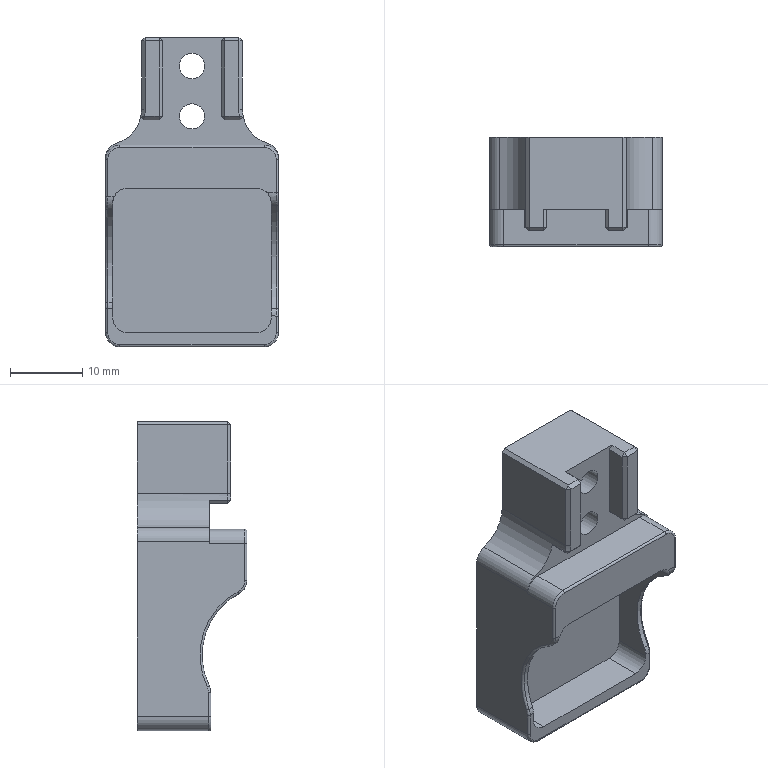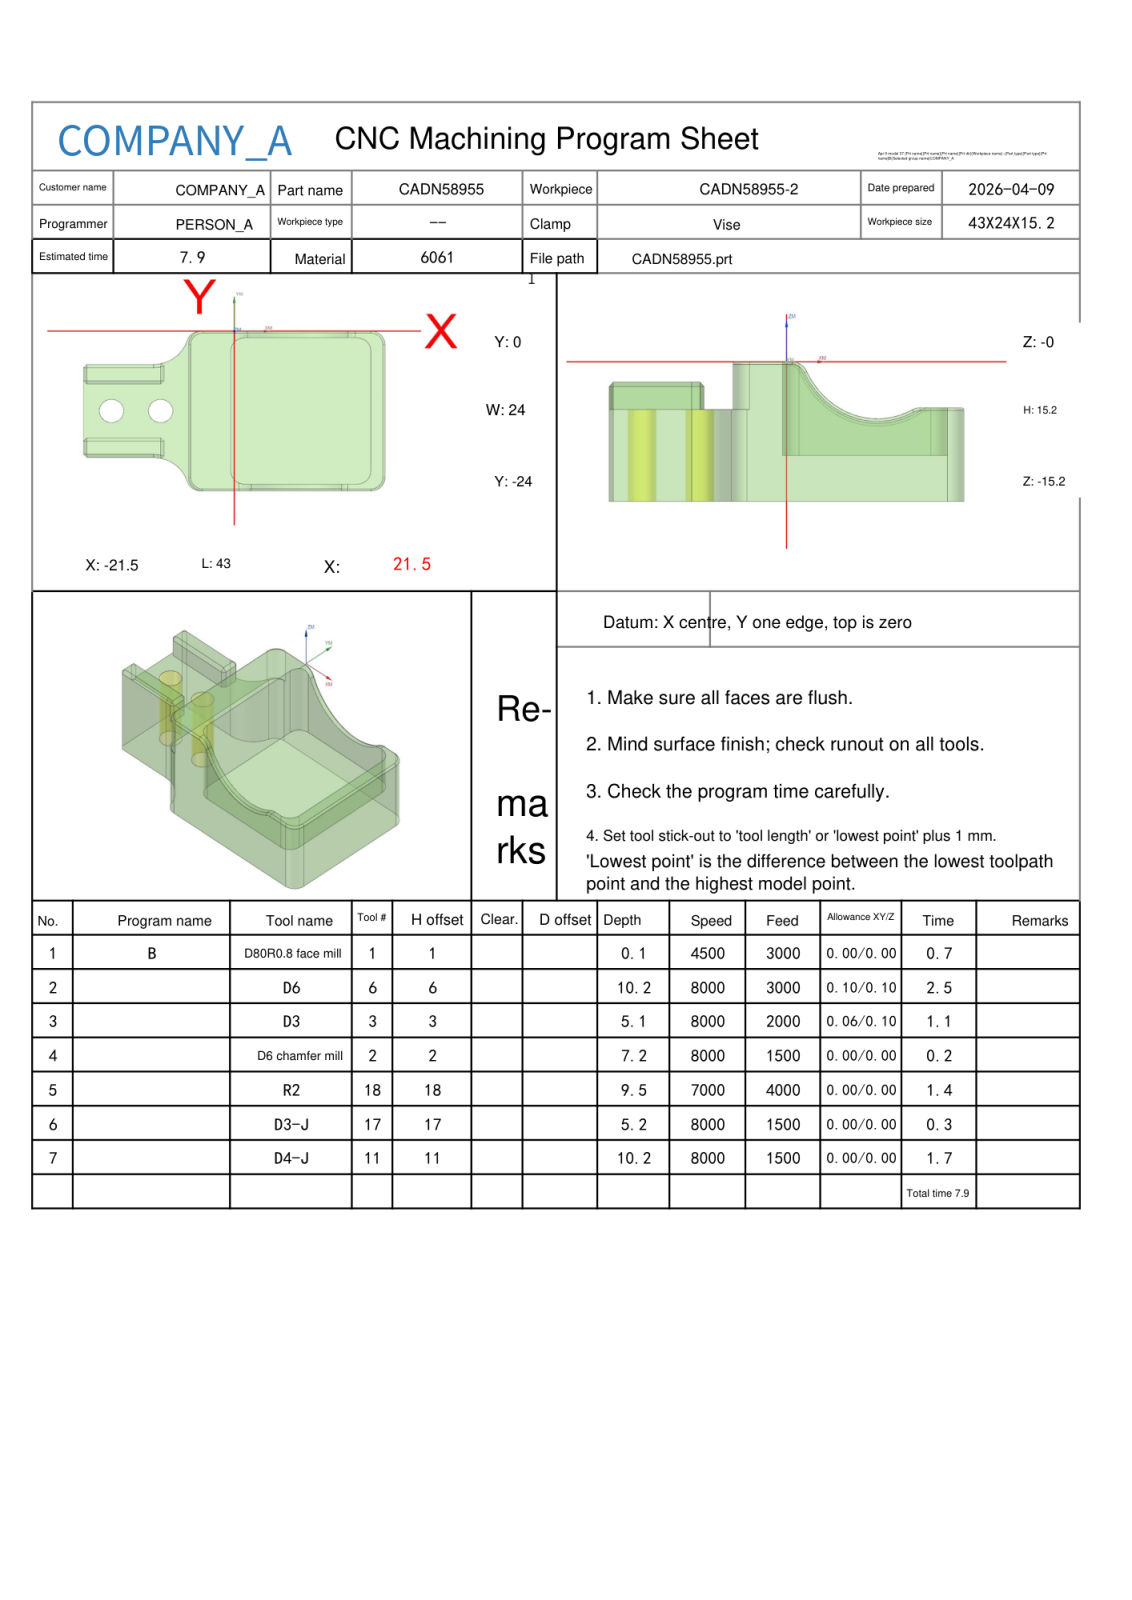NC program | NX | posted by the shop | part box 24 x 15.2 x 43 mm
Lines 3234 to 4724 of 14472:
N5 T18 M06
(R2  D=4. R=2. H=18 ce=0.01 di=0.00)
G00 G90 G54 X3.945 Y-24.084 M03 S7000
G43 H18 Z14.5
M08
Z.491
G01 Z-.009 F4000.
X1.773 Y-23.864
X1.579 Y-23.845
X.675 Y-23.917
X-4.5
G02 X-6.417 Y-22. I0.0 J1.917
G01 Y-2.
G02 X-4.5 Y-.083 I1.917 J0.0
G01 X.099
X1.018 Y-.155
X1.197 Y-.136
X1.199 Y-.039 Z-.016
Y.003 Z-.022
X.175 Y.009
X.099 Y.028
X-4.5
G03 X-6.528 Y-2. I0.0 J-2.028
G01 Y-22.
G03 X-4.5 Y-24.028 I2.028 J0.0
G01 X.675
X.737 Y-24.01
X1.774 Y-23.998
Y-24.071 Z-.031
Y-24.091 Z-.039
X.737 Y-24.103
X.675 Y-24.132
X-4.5
G02 X-6.632 Y-22. I0.0 J2.132
G01 Y-2.
G02 X-4.5 Y.132 I2.132 J0.0
G01 X.099
X.175 Y.103
X1.199 Y.1
Y.174 Z-.05
Y.216 Z-.06
X.175 Y.22
X.099 Y.233
X-4.5
G03 X-6.733 Y-2. I0.0 J-2.233
G01 Y-22.
G03 X-4.5 Y-24.233 I2.233 J0.0
G01 X.675
X.737 Y-24.22
X1.774 Y-24.208
Y-24.275 Z-.073
Y-24.313 Z-.086
X.737 Y-24.32
X.675 Y-24.333
X-4.5
G02 X-6.833 Y-22. I0.0 J2.333
G01 Y-2.
G02 X-4.5 Y.333 I2.333 J0.0
G01 X.099
X.175 Y.32
X1.199 Y.312
Y.374 Z-.101
Y.406 Z-.116
X.175 Y.414
X.099 Y.43
X-4.5
G03 X-6.93 Y-2. I0.0 J-2.43
G01 Y-22.
G03 X-4.5 Y-24.43 I2.43 J0.0
G01 X.675
X.737 Y-24.414
X1.774 Y-24.407
Y-24.471 Z-.133
Y-24.513 Z-.149
X.737 Y-24.52
X.675 Y-24.526
X-4.5
G02 X-7.026 Y-22. I0.0 J2.526
G01 Y-2.
G02 X-4.5 Y.526 I2.526 J0.0
G01 X.099
X.175 Y.52
X1.199 Y.512
Y.568 Z-.168
Y.603 Z-.187
X.175 Y.609
X.099 Y.619
X-4.5
G03 X-7.119 Y-2. I0.0 J-2.619
G01 Y-22.
G03 X-4.5 Y-24.619 I2.619 J0.0
G01 X.675
X.737 Y-24.609
X1.774 Y-24.604
Y-24.661 Z-.208
Y-24.692 Z-.229
X.737 Y-24.698
X.675 Y-24.711
X-4.5
G02 X-7.211 Y-22. I0.0 J2.711
G01 Y-2.
G02 X-4.5 Y.711 I2.711 J0.0
G01 X.099
X.175 Y.697
X1.199 Y.691
Y.75 Z-.252
Y.788 Z-.275
X1.018 Y.791
X.175 Y.793
X.099 Y.801
X-4.5
G03 X-7.301 Y-2. I0.0 J-2.801
G01 Y-22.
G03 X-4.5 Y-24.801 I2.801 J0.0
G01 X.675
X.737 Y-24.794
X1.774 Y-24.788
X1.719 Y-24.881 Z-.325
X.737 Y-24.879
X.675 Y-24.888
X-4.5
G02 X-7.388 Y-22. I0.0 J2.888
G01 Y-2.
G02 X-4.5 Y.888 I2.888 J0.0
G01 X.099
X.175 Y.884
X1.018 Y.882
X1.199 Y.879
Y.929 Z-.351
X1.2 Y.968 Z-.378
X1.018 Y.971
X.099 Y.973
X-4.5
G03 X-7.473 Y-2. I0.0 J-2.973
G01 Y-22.
G03 X-4.5 Y-24.973 I2.973 J0.0
G01 X.675
X1.779 Y-24.971
X1.788 Y-25.012 Z-.407
X1.798 Y-25.054 Z-.435
X.737 Y-25.047
X.675 Y-25.056
X-4.5
G02 X-7.556 Y-22. I0.0 J3.056
G01 Y-2.
G02 X-4.5 Y1.056 I3.056 J0.0
G01 X.099
X.175 Y1.052
X1.018 Y1.051
X1.199 Y1.048
Y1.094 Z-.465
Y1.132 Z-.495
X.175 Y1.133
X.099 Y1.136
X-4.5
G03 X-7.636 Y-2. I0.0 J-3.136
G01 Y-22.
G03 X-4.5 Y-25.136 I3.136 J0.0
G01 X.675
X.737 Y-25.133
X1.774
Y-25.172 Z-.527
Y-25.209 Z-.559
X.675 Y-25.213
X-4.5
G02 X-7.713 Y-22. I0.0 J3.213
G01 Y-2.
G02 X-4.5 Y1.213 I3.213 J0.0
G01 X.099
X.175 Y1.21
X1.202 Y1.208
X1.201 Y1.249 Z-.593
X1.199 Y1.285 Z-.627
X1.177 Y1.284
X.175 Y1.285
X.099 Y1.288
X-4.5
G03 X-7.788 Y-2. I0.0 J-3.288
G01 Y-22.
G03 X-4.5 Y-25.288 I3.288 J0.0
G01 X.675
X.737 Y-25.285
X1.7 Y-25.284
X1.784 Y-25.281
X1.779 Y-25.323 Z-.662
X1.775 Y-25.357 Z-.697
X1.712 Y-25.355
X.737 Y-25.356
X.675 Y-25.359
X-4.5
G02 X-7.859 Y-22. I0.0 J3.359
G01 Y-2.
G02 X-4.5 Y1.359 I3.359 J0.0
G01 X.099
X.175 Y1.356
X1.199
Y1.391 Z-.734
Y1.424 Z-.77
X1.125 Y1.423
X.175 Y1.424
X.099 Y1.428
X-4.5
G03 X-7.928 Y-2. I0.0 J-3.428
G01 Y-22.
G03 X-4.5 Y-25.428 I3.428 J0.0
G01 X.675
X.737 Y-25.425
X1.775 Y-25.423
Y-25.457 Z-.808
Y-25.487 Z-.847
X.737 Y-25.489
X.675 Y-25.493
X-4.5
G02 X-7.993 Y-22. I0.0 J3.493
G01 Y-2.
G02 X-4.5 Y1.493 I3.493 J0.0
G01 X.099
X.175 Y1.489
X1.199 Y1.488
Y1.521 Z-.886
Y1.551 Z-.926
X1.142 Y1.55
X.175 Y1.551
X.099 Y1.554
X-4.5
G03 X-8.054 Y-2. I0.0 J-3.554
G01 Y-22.
G03 X-4.5 Y-25.554 I3.554 J0.0
G01 X.675
X.737 Y-25.551
X1.704 Y-25.55
X1.775 Y-25.552
Y-25.582 Z-.966
Y-25.607 Z-1.007
X1.712 Y-25.606
X.737 Y-25.607
X.675 Y-25.612
X-4.5
G02 X-8.112 Y-22. I0.0 J3.612
G01 Y-2.
G02 X-4.5 Y1.612 I3.612 J0.0
G01 X.099
X.175 Y1.607
X1.15 Y1.606
X1.199 Y1.607
Y1.639 Z-1.049
X1.2 Y1.664 Z-1.091
X.175 Y1.665
X.099 Y1.667
X-4.5
G03 X-8.167 Y-2. I0.0 J-3.667
G01 Y-22.
G03 X-4.5 Y-25.667 I3.667 J0.0
G01 X.675
X.737 Y-25.665
X1.775 Y-25.664
Y-25.691 Z-1.134
X1.774 Y-25.713 Z-1.177
X1.7 Y-25.711
X.737 Y-25.713
X.675 Y-25.717
X-4.5
G02 X-8.217 Y-22. I0.0 J3.717
G01 Y-2.
G02 X-4.5 Y1.717 I3.717 J0.0
G01 X.099
X.175 Y1.712
X1.2 Y1.714
Y1.738 Z-1.222
Y1.761 Z-1.266
X.175 Y1.759
X.099 Y1.764
X-4.5
G03 X-8.264 Y-2. I0.0 J-3.764
G01 Y-22.
G03 X-4.5 Y-25.764 I3.764 J0.0
G01 X.675
X.737 Y-25.759
X1.775 Y-25.758
Y-25.785 Z-1.311
Y-25.803 Z-1.356
X1.708 Y-25.804
X.737 Y-25.806
X.675 Y-25.807
X-4.5
G02 X-8.307 Y-22. I0.0 J3.807
G01 Y-2.
G02 X-4.5 Y1.807 I3.807 J0.0
G01 X.099
X.175 Y1.806
X1.2 Y1.805
Y1.824 Z-1.402
Y1.842 Z-1.448
X1.154 Y1.843
X.175 Y1.844
X.099 Y1.847
X-4.5
G03 X-8.347 Y-2. I0.0 J-3.847
G01 Y-22.
G03 X-4.5 Y-25.847 I3.847 J0.0
G01 X.675
X.737 Y-25.844
X1.711 Y-25.843
X1.775
Y-25.863 Z-1.495
Y-25.878 Z-1.542
X.737 Y-25.88
X.675 Y-25.882
X-4.5
G02 X-8.382 Y-22. I0.0 J3.882
G01 Y-2.
G02 X-4.5 Y1.882 I3.882 J0.0
G01 X.099
X.175 Y1.88
X1.158 Y1.879
X1.2 Y1.878
Y1.894 Z-1.59
Y1.907 Z-1.637
X1.156 Y1.908
X.175
X.099 Y1.912
X-4.5
G03 X-8.412 Y-2. I0.0 J-3.912
G01 Y-22.
G03 X-4.5 Y-25.912 I3.912 J0.0
G01 X.675
X.737 Y-25.908
X1.717
X1.775
Y-25.922 Z-1.685
Y-25.935 Z-1.734
X.737 Y-25.936
X.675 Y-25.939
X-4.5
G02 X-8.439 Y-22. I0.0 J3.939
G01 Y-2.
G02 X-4.5 Y1.939 I3.939 J0.0
G01 X.099
X.175 Y1.935
X1.158 Y1.934
X1.2
X1.201 Y1.949 Z-1.782
X1.202 Y1.96 Z-1.831
X.175 Y1.961
X.099 Y1.962
X-4.5
G03 X-8.462 Y-2. I0.0 J-3.962
G01 Y-22.
G03 X-4.5 Y-25.962 I3.962 J0.0
G01 X.675
X.737 Y-25.961
X1.781 Y-25.96
Y-25.97 Z-1.88
Y-25.978 Z-1.929
X.737 Y-25.979
X.675 Y-25.98
X-4.5
G02 X-8.48 Y-22. I0.0 J3.98
G01 Y-2.
G02 X-4.5 Y1.98 I3.98 J0.0
G01 X.099
X.175 Y1.979
X1.202 Y1.978
Y1.984 Z-1.976
Y1.989 Z-2.022
X.175
X.099 Y1.993
X-4.5
G03 X-8.493 Y-2. I0.0 J-3.993
G01 Y-22.
G03 X-4.5 Y-25.993 I3.993 J0.0
G01 X.675
X.737 Y-25.989
X1.781
Y-25.997 Z-2.115
X.737 Y-25.998
X.675 Y-26.003
X-4.5
G02 X-8.503 Y-22. I0.0 J4.003
G01 Y-2.
G02 X-4.5 Y2.003 I4.003 J0.0
G01 X.099
X.175 Y1.998
X1.202 Y1.997
Y2.006 Z-2.207
X.175
X.099 Y2.008
X-4.5
G03 X-8.508 Y-2. I0.0 J-4.008
G01 Y-22.
G03 X-4.5 Y-26.008 I4.008 J0.0
G01 X.675
X.737 Y-26.006
X1.781
Y-26.01 Z-2.3
X-4.529 Y-26.009
G02 X-4.744 Y-26.003 I0.0 J3.532
X-8.25 Y-23.42 I.244 J4.003
X-8.51 Y-22. I3.75 J1.42
G01 Y-2.
G02 X-8.25 Y-.58 I4.01 J0.0
X-4.878 Y1.992 I3.75 J-1.42
G01 X-4.5 Y2.01
X1.202
G00 Z14.5
G00 G90 X13.988 Y-.296 M03 S7000
Z14.5
Z-4.509
G01 Z-5.009 F4000.
X16.131 Y-.155
X17.231 Y-.083
X19.5
G02 X21.417 Y-2. I0.0 J-1.917
G01 Y-22.
G02 X19.5 Y-23.917 I-1.917 J0.0
G01 X16.159
X15.277 Y-23.845
X15.063 Y-23.878
X15.06 Y-23.961 Z-5.016
X15.059 Y-24. Z-5.022
X16.123 Y-24.013
X16.159 Y-24.028
X19.5
G03 X21.528 Y-22. I0.0 J2.028
G01 Y-2.
G03 X19.5 Y.028 I-2.028 J0.0
G01 X17.231
X16.131 Y.004
Y.07 Z-5.031
Y.098 Z-5.039
X17.231 Y.132
X19.5
G02 X21.632 Y-2. I0.0 J-2.132
G01 Y-22.
G02 X19.5 Y-24.132 I-2.132 J0.0
G01 X16.159
X15.059 Y-24.093
Y-24.21 Z-5.06
X16.123 Y-24.222
X16.159 Y-24.233
X19.5
G03 X21.733 Y-22. I0.0 J2.233
G01 Y-2.
G03 X19.5 Y.233 I-2.233 J0.0
G01 X17.231
X16.131 Y.215
Y.275 Z-5.073
Y.317 Z-5.086
X17.231 Y.333
X19.5
G02 X21.833 Y-2. I0.0 J-2.333
G01 Y-22.
G02 X19.5 Y-24.333 I-2.333 J0.0
G01 X16.159
X16.123 Y-24.321
X15.108
X15.03 Y-24.32
X15.057 Y-24.42 Z-5.116
X15.104 Y-24.412
X16.123 Y-24.414
X16.159 Y-24.43
X19.5
G03 X21.93 Y-22. I0.0 J2.43
G01 Y-2.
G03 X19.5 Y.43 I-2.43 J0.0
G01 X17.231
X16.131 Y.411
Y.471 Z-5.133
Y.517 Z-5.149
X17.231 Y.526
X19.5
G02 X22.026 Y-2. I0.0 J-2.526
G01 Y-22.
G02 X19.5 Y-24.526 I-2.526 J0.0
G01 X16.159
X16.123 Y-24.521
X15.05 Y-24.52
X15.055 Y-24.571 Z-5.168
X15.059 Y-24.616 Z-5.187
X16.159 Y-24.619
X19.5
G03 X22.119 Y-22. I0.0 J2.619
G01 Y-2.
G03 X19.5 Y.619 I-2.619 J0.0
G01 X17.231
X16.131 Y.607
Y.661 Z-5.208
Y.695 Z-5.229
X17.231 Y.711
X19.5
G02 X22.211 Y-2. I0.0 J-2.711
G01 Y-22.
G02 X19.5 Y-24.711 I-2.711 J0.0
G01 X16.159
X16.123 Y-24.698
X15.059 Y-24.707
X15.055 Y-24.753 Z-5.252
X15.051 Y-24.796 Z-5.275
X16.123 Y-24.795
X16.159 Y-24.801
X19.5
G03 X22.301 Y-22. I0.0 J2.801
G01 Y-2.
G03 X19.5 Y.801 I-2.801 J0.0
G01 X17.231
X16.131 Y.791
Y.84 Z-5.3
Y.884 Z-5.325
X16.161 Y.882
X17.231 Y.888
X19.5
G02 X22.388 Y-2. I0.0 J-2.888
G01 Y-22.
G02 X19.5 Y-24.888 I-2.888 J0.0
G01 X16.159
X16.123 Y-24.88
X15.045 Y-24.882
Y-24.927 Z-5.351
Y-24.971 Z-5.378
X16.123 Y-24.961
X16.159 Y-24.973
X19.5
G03 X22.473 Y-22. I0.0 J2.973
G01 Y-2.
G03 X19.5 Y.973 I-2.973 J0.0
G01 X17.231
X16.123 Y.971
X16.127 Y1.014 Z-5.407
X16.131 Y1.052 Z-5.435
X17.231 Y1.056
X19.5
G02 X22.556 Y-2. I0.0 J-3.056
G01 Y-22.
G02 X19.5 Y-25.056 I-3.056 J0.0
G01 X16.159
X16.123 Y-25.048
X15.045 Y-25.051
X15.053 Y-25.094 Z-5.465
X15.059 Y-25.133 Z-5.495
X16.123 Y-25.134
X16.159 Y-25.136
X19.5
G03 X22.636 Y-22. I0.0 J3.136
G01 Y-2.
G03 X19.5 Y1.136 I-3.136 J0.0
G01 X17.231
X16.131 Y1.132
Y1.171 Z-5.527
Y1.209 Z-5.559
X17.231 Y1.213
X19.5
G02 X22.713 Y-2. I0.0 J-3.213
G01 Y-22.
G02 X19.5 Y-25.213 I-3.213 J0.0
G01 X16.159
X16.123 Y-25.211
X15.056 Y-25.208
X15.058 Y-25.249 Z-5.593
X15.059 Y-25.285 Z-5.627
X15.081 Y-25.284
X16.123 Y-25.285
X16.159 Y-25.288
X19.5
G03 X22.788 Y-22. I0.0 J3.288
G01 Y-2.
G03 X19.5 Y1.288 I-3.288 J0.0
G01 X17.231
X16.14 Y1.281
X16.131 Y1.285
Y1.323 Z-5.662
Y1.357 Z-5.697
X16.193 Y1.355
X17.231 Y1.359
X19.5
G02 X22.859 Y-2. I0.0 J-3.359
G01 Y-22.
G02 X19.5 Y-25.359 I-3.359 J0.0
G01 X16.159
X16.123 Y-25.357
X15.059 Y-25.355
Y-25.391 Z-5.734
Y-25.424 Z-5.77
X16.123 Y-25.425
X16.159 Y-25.428
X19.5
G03 X22.928 Y-22. I0.0 J3.428
G01 Y-2.
G03 X19.5 Y1.428 I-3.428 J0.0
G01 X17.231
X16.131 Y1.423
Y1.457 Z-5.808
Y1.487 Z-5.847
X17.231 Y1.493
X19.5
G02 X22.993 Y-2. I0.0 J-3.493
G01 Y-22.
G02 X19.5 Y-25.493 I-3.493 J0.0
G01 X16.159
X16.123 Y-25.489
X15.059
Y-25.52 Z-5.886
Y-25.551 Z-5.926
X16.123 Y-25.552
X16.159 Y-25.554
X19.5
G03 X23.054 Y-22. I0.0 J3.554
G01 Y-2.
G03 X19.5 Y1.554 I-3.554 J0.0
G01 X17.231
X16.131 Y1.55
Y1.581 Z-5.966
Y1.606 Z-6.007
X17.231 Y1.612
X19.5
G02 X23.112 Y-2. I0.0 J-3.612
G01 Y-22.
G02 X19.5 Y-25.612 I-3.612 J0.0
G01 X16.159
X16.123 Y-25.608
X15.059 Y-25.609
Y-25.637 Z-6.049
Y-25.664 Z-6.091
X16.159 Y-25.667
X19.5
G03 X23.167 Y-22. I0.0 J3.667
G01 Y-2.
G03 X19.5 Y1.667 I-3.667 J0.0
G01 X17.231
X16.131 Y1.664
Y1.689 Z-6.134
Y1.711 Z-6.177
X17.231 Y1.717
X19.5
G02 X23.217 Y-2. I0.0 J-3.717
G01 Y-22.
G02 X19.5 Y-25.717 I-3.717 J0.0
G01 X16.159
X16.123 Y-25.713
X15.059 Y-25.712
Y-25.739 Z-6.222
Y-25.758 Z-6.266
X16.123 Y-25.759
X16.159 Y-25.764
X19.5
G03 X23.264 Y-22. I0.0 J3.764
G01 Y-2.
G03 X19.5 Y1.764 I-3.764 J0.0
G01 X17.231
X16.131 Y1.757
Y1.783 Z-6.311
Y1.804 Z-6.356
X17.231 Y1.807
X19.5
G02 X23.307 Y-2. I0.0 J-3.807
G01 Y-22.
G02 X19.5 Y-25.807 I-3.807 J0.0
G01 X16.159
X16.123 Y-25.806
X15.058 Y-25.805
Y-25.824 Z-6.402
Y-25.843 Z-6.448
X16.123 Y-25.844
X16.159 Y-25.847
X19.5
G03 X23.347 Y-22. I0.0 J3.847
G01 Y-2.
G03 X19.5 Y1.847 I-3.847 J0.0
G01 X17.231
X16.131 Y1.843
Y1.861 Z-6.495
Y1.879 Z-6.542
X17.231 Y1.882
X19.5
G02 X23.382 Y-2. I0.0 J-3.882
G01 Y-22.
G02 X19.5 Y-25.882 I-3.882 J0.0
G01 X16.159
X15.277 Y-25.879
X15.058
Y-25.894 Z-6.59
X15.059 Y-25.908 Z-6.637
X16.123 Y-25.909
X16.159 Y-25.912
X19.5
G03 X23.412 Y-22. I0.0 J3.912
G01 Y-2.
G03 X19.5 Y1.912 I-3.912 J0.0
G01 X17.231
X16.131 Y1.908
Y1.922 Z-6.685
Y1.934 Z-6.734
X17.231 Y1.939
X19.5
G02 X23.439 Y-2. I0.0 J-3.939
G01 Y-22.
G02 X19.5 Y-25.939 I-3.939 J0.0
G01 X16.159
X16.123 Y-25.936
X15.059
X15.058 Y-25.949 Z-6.782
X15.057 Y-25.96 Z-6.831
X16.123 Y-25.961
X16.159 Y-25.962
X19.5
G03 X23.462 Y-22. I0.0 J3.962
G01 Y-2.
G03 X19.5 Y1.962 I-3.962 J0.0
G01 X17.231
X16.132 Y1.96
Y1.97 Z-6.88
Y1.978 Z-6.929
X17.231 Y1.98
X19.5
G02 X23.48 Y-2. I0.0 J-3.98
G01 Y-22.
G02 X19.5 Y-25.98 I-3.98 J0.0
G01 X16.159
X16.123 Y-25.979
X15.057 Y-25.978
Y-25.984 Z-6.976
Y-25.989 Z-7.022
X16.123
X16.159 Y-25.993
X19.5
G03 X23.493 Y-22. I0.0 J3.993
G01 Y-2.
G03 X19.5 Y1.993 I-3.993 J0.0
G01 X17.231
X16.132 Y1.99
Y1.999 Z-7.115
X17.231 Y2.003
X19.5
G02 X23.503 Y-2. I0.0 J-4.003
G01 Y-22.
G02 X19.5 Y-26.003 I-4.003 J0.0
G01 X16.159
X16.123 Y-25.998
X15.057 Y-25.997
Y-26.006 Z-7.207
X16.123
X16.159 Y-26.008
X19.5
G03 X23.508 Y-22. I0.0 J4.008
G01 Y-2.
G03 X19.5 Y2.008 I-4.008 J0.0
G01 X17.231
X16.132 Y2.007
Y2.009 Z-7.3
X19.508 Y2.01
G02 X23.51 Y-2. I-.008 J-4.01
G01 Y-22.
G02 X19.508 Y-26.01 I-4.01 J0.0
G01 X15.057
G00 Z14.5
G00 G90 X.164 Y-22.174 M03 S7000
Z20.
Z7.997
G01 Z-.003 F3500.
X.432
X.539 Y-22.214 Z-.005
X.741 Y-22.274 Z-.007
X.45 Z-.002
X.165 Z-.001
Y-22.371 Z0.0
X.54 Z-.003
X.848 Z-.009
X1.048 Z-.024
X1.172 Y-22.37 Z-.039
X1.247 Y-22.386 Z-.049
X1.517 Y-22.422 Z-.102
X1.645 Y-22.439 Z-.133
X1.845 Y-22.454 Z-.192
X2.044 Y-22.468 Z-.262
X2.113 Y-22.47 Z-.289
X2.045 Z-.262
X1.845 Z-.192
X1.645 Z-.132
X1.542 Z-.107
X1.247 Z-.048
X1.048 Z-.023
X.848 Z-.008
X.45 Z-.001
X.166 Z0.0
Z8.
G00 X3.417 Y-22.469
Z6.866
G01 Z-1.134
X3.439 Z-1.153
X3.543 Z-1.264
X3.638 Z-1.361
X3.838 Z-1.604
X4.037 Z-1.89
X4.435 Z-2.534
X4.843 Y-22.468 Z-3.117
X4.938 Z-3.243
X5.232 Z-3.591
X5.641 Z-4.016
X6.04 Z-4.376
X6.428 Z-4.686
X6.827 Z-4.967
X7.037 Y-22.467 Z-5.097
X7.225 Z-5.201
X7.624 Z-5.41
X7.812 Z-5.505
X8.022 Z-5.598
X8.421 Z-5.745
X8.82 Z-5.876
X9.218 Z-5.986
X9.804 Y-22.466 Z-6.102
X10.015 Z-6.132
X10.414 Z-6.17
X10.812 Z-6.18
X11.211 Z-6.183
X11.609 Z-6.168
X12.008 Y-22.465 Z-6.129
X12.407 Z-6.062
X12.805 Z-5.976
X13.204 Z-5.874
X13.416 Z-5.808
X14.001 Y-22.464 Z-5.592
X14.43 Z-5.412
X14.477 Z-5.394
X14.799 Y-22.47 Z-5.271
X14.894 Y-22.472 Z-5.237
X15.098 Y-22.476 Z-5.171
X15.196 Y-22.478 Z-5.141
X15.396 Y-22.484 Z-5.094
X15.595 Y-22.489 Z-5.06
X15.994 Y-22.502 Z-5.011
X16.392 Y-22.522 Z-5.
X16.668 Y-22.546 Z-5.002
X16.674 Y-22.547
X16.678 Y-22.556
X16.679 Y-22.562
X16.392 Y-22.563 Z-5.
X15.994 Z-5.01
X15.82 Z-5.029
X15.595 Z-5.057
X15.396 Z-5.091
X15.196 Z-5.138
X15.053 Z-5.18
X14.941 Z-5.217
X14.799 Z-5.267
X14.574 Z-5.353
X14.399 Z-5.423
X14.001 Y-22.564 Z-5.591
X13.602 Z-5.738
X13.426 Z-5.797
X13.315 Z-5.839
X13.204 Z-5.873
X12.805 Z-5.975
X12.407 Z-6.061
X12.008 Z-6.128
X11.609 Y-22.565 Z-6.166
X11.211 Z-6.183
X10.812 Z-6.18
X10.414 Z-6.169
X10.015 Z-6.131
X9.905 Z-6.116
X9.796 Z-6.094
X9.617 Z-6.064
X9.218 Y-22.566 Z-5.985
X8.82 Z-5.875
X8.421 Z-5.744
X8.022 Z-5.597
X7.913 Z-5.549
X7.805 Z-5.494
X7.624 Z-5.409
X7.225 Z-5.2
X7.044 Y-22.567 Z-5.093
X6.935 Z-5.033
X6.827 Z-4.966
X6.428 Z-4.685
X6.337 Z-4.616
X6.121 Z-4.444
X5.938 Z-4.29
X5.722 Z-4.094
X5.54 Z-3.914
X5.324 Z-3.689
X5.232 Z-3.59
X5.141 Z-3.48
X5.049 Z-3.365
X4.888 Y-22.568 Z-3.174
X4.834 Z-3.103
X4.435 Z-2.53
X4.037 Z-1.885
X3.838 Z-1.599
X3.638 Z-1.355
X3.439 Z-1.148
X3.24 Z-.967
X3.04 Z-.807
X2.841 Z-.667
X2.642 Z-.542
X2.443 Y-22.569 Z-.432
X2.243 Z-.337
X2.044 Z-.258
X1.845 Z-.189
X1.645 Z-.13
X1.592 Z-.117
X1.247 Z-.047
X1.048 Z-.022
X.848 Z-.007
X.45 Z0.0
X.167 Y-22.57
X.168 Y-22.669
X.45
X.848 Z-.007
X1.048 Z-.022
X1.247 Z-.046
X1.645 Z-.127
X1.845 Z-.186
X2.044 Z-.255
X2.243 Z-.333
X2.443 Y-22.668 Z-.428
X2.642 Z-.538
X2.841 Z-.662
X3.04 Z-.802
X3.24 Z-.961
X3.439 Z-1.142
X3.638 Z-1.351
X3.838 Z-1.594
X4.037 Z-1.88
X4.446 Z-2.541
X4.64 Y-22.667 Z-2.826
X4.845 Z-3.115
X5.039 Z-3.358
X5.232 Z-3.589
X5.437 Z-3.811
X5.631 Z-4.005
X5.836 Z-4.203
X6.235 Z-4.539
X6.428 Z-4.684
X6.839 Z-4.973
X7.225 Y-22.666 Z-5.2
X7.624 Z-5.409
X8.022 Z-5.597
X8.421 Z-5.744
X8.82 Z-5.875
X9.218 Y-22.665 Z-5.984
X9.617 Z-6.064
X10.015 Z-6.131
X10.43 Z-6.169
X10.812 Z-6.181
X11.227 Z-6.183
X11.609 Y-22.664 Z-6.165
X12.008 Z-6.127
X12.407 Z-6.061
X12.805 Z-5.975
X13.213 Z-5.87
X13.602 Z-5.737
X14.001 Y-22.663 Z-5.591
X14.399 Z-5.423
X14.798 Z-5.263
X15.002 Z-5.192
X15.196 Z-5.134
X15.396 Z-5.087
X15.615 Z-5.051
X15.994 Z-5.01
X16.392 Y-22.662 Z-5.
X16.677 Z-5.002
X16.675 Y-22.762
X16.392 Z-5.
X15.994 Z-5.009
X15.948 Z-5.012
X15.595 Y-22.763 Z-5.051
X15.442 Z-5.077
X15.35 Z-5.096
X15.196 Z-5.132
X14.997 Z-5.19
X14.798 Z-5.26
X14.706 Z-5.299
X14.399 Z-5.423
X14.307 Z-5.464
X14.001 Z-5.593
X13.602 Z-5.741
X13.204 Y-22.764 Z-5.876
X12.805 Z-5.979
X12.407 Z-6.064
X12.008 Z-6.131
X11.609 Z-6.169
X11.211 Z-6.186
X10.812 Y-22.765 Z-6.183
X10.602 Z-6.176
X10.461
X10.015 Z-6.134
X9.617 Z-6.067
X9.218 Z-5.988
X8.82 Z-5.879
X8.421 Y-22.766 Z-5.748
X8.022 Z-5.6
X7.624 Z-5.413
X7.225 Z-5.204
X6.827 Z-4.97
X6.428 Y-22.767 Z-4.689
X6.229 Z-4.54
X5.83 Z-4.203
X5.631 Z-4.01
X5.432 Z-3.81
X5.232 Z-3.595
X5.033 Z-3.356
X4.834 Z-3.107
X4.635 Z-2.824
X4.435 Z-2.529
X4.339 Z-2.363
X4.037 Y-22.768 Z-1.874
X3.838 Z-1.589
X3.638 Z-1.346
X3.439 Z-1.137
X3.24 Z-.957
X3.04 Z-.799
X2.841 Z-.659
X2.642 Z-.535
X2.443 Z-.426
X2.243 Z-.332
X2.044 Z-.253
X1.845 Y-22.769 Z-.184
X1.645 Z-.126
X1.247 Z-.045
X1.048 Z-.021
X.848 Z-.006
X.45 Z0.0
X.169
X.17 Y-22.869
X.45
X.848 Z-.006
X1.048 Z-.021
X1.247 Y-22.868 Z-.045
X1.645 Z-.125
X1.845 Z-.183
X2.044 Z-.251
X2.243 Z-.33
X2.443 Z-.424
X2.642 Z-.532
X2.841 Z-.655
X3.04 Z-.795
X3.24 Z-.953
X3.439 Z-1.133
X3.638 Y-22.867 Z-1.341
X3.838 Z-1.583
X4.037 Z-1.868
X4.237 Z-2.192
X4.435 Z-2.533
X4.635 Z-2.829
X4.834 Z-3.114
X5.033 Z-3.362
X5.232 Z-3.601
X5.432 Z-3.816
X5.631 Z-4.016
X5.83 Y-22.866 Z-4.208
X6.229 Z-4.545
X6.428 Z-4.693
X6.827 Z-4.975
X7.225 Z-5.208
X7.624 Z-5.417
X8.022 Z-5.604
X8.421 Y-22.865 Z-5.752
X8.82 Z-5.883
X9.218 Z-5.992
X9.617 Z-6.071
X10.015 Z-6.138
X10.512 Y-22.864 Z-6.184
X11.211 Z-6.189
X11.406 Z-6.182
X11.609 Z-6.172
X12.008 Z-6.135
X12.407 Z-6.068
X12.805 Y-22.863 Z-5.983
X13.204 Z-5.88
X13.602 Z-5.744
X13.806 Z-5.669
X14.001 Z-5.595
X14.205 Z-5.509
X14.399 Z-5.422
X14.604 Z-5.34
X14.798 Z-5.257
X14.997 Z-5.188
X15.196 Y-22.862 Z-5.13
X15.299 Z-5.106
X15.493 Z-5.066
X15.595 Z-5.049
X15.897 Z-5.015
X15.994 Z-5.008
X16.392 Z-5.
X16.673 Z-5.001
X16.672 Y-22.961 Z-5.
X16.392 Y-22.962
X15.994 Z-5.007
X15.846 Z-5.018
X15.595 Z-5.047
X15.544 Z-5.056
X15.248 Z-5.116
X15.196 Z-5.128
X14.997 Z-5.185
X14.798 Z-5.253
X14.502 Z-5.38
X14.399 Z-5.421
X14.103 Y-22.963 Z-5.554
X14.001 Z-5.597
X13.602 Z-5.748
X13.204 Z-5.884
X12.805 Z-5.987
X12.407 Z-6.072
X12.008 Z-6.138
X11.609 Y-22.964 Z-6.176
X11.407 Z-6.184
X11.309 Z-6.192
X11.211 Z-6.197
X10.563 Z-6.192
X10.015 Z-6.141
X9.617 Y-22.965 Z-6.075
X9.218 Z-5.996
X8.82 Z-5.887
X8.421 Z-5.756
X8.022 Z-5.609
X7.624 Z-5.421
X7.225 Y-22.966 Z-5.212
X6.827 Z-4.98
X6.428 Z-4.698
X6.229 Z-4.55
X5.83 Z-4.213
X5.631 Z-4.021
X5.432 Z-3.821
X5.232 Z-3.607
X5.033 Y-22.967 Z-3.368
X4.834 Z-3.12
X4.635 Z-2.835
X4.435 Z-2.536
X4.135 Z-2.021
X4.037 Z-1.862
X3.838 Z-1.578
X3.638 Z-1.336
X3.439 Z-1.129
X3.24 Z-.949
X3.04 Z-.791
X2.841 Z-.652
X2.642 Y-22.968 Z-.529
X2.443 Z-.422
X2.243 Z-.329
X2.044 Z-.25
X1.845 Z-.182
X1.645 Z-.125
X1.247 Z-.044
X1.048 Z-.021
X.848 Z-.006
X.45 Z0.0
X.171 Y-22.969
X.172 Y-23.068
X.45
X.848 Z-.005
X1.05 Z-.021
X1.247 Z-.044
X1.645 Y-23.067 Z-.124
X1.845 Z-.18
X2.044 Z-.248
X2.243 Z-.327
X2.443 Z-.42
X2.642 Z-.526
X2.841 Z-.648
X3.04 Z-.787
X3.24 Z-.945
X3.439 Z-1.124
X3.638 Y-23.066 Z-1.332
X3.838 Z-1.572
X4.037 Z-1.856
X4.435 Z-2.539
X4.635 Z-2.84
X4.834 Z-3.125
X5.033 Z-3.374
X5.232 Z-3.612
X5.433 Z-3.828
X5.631 Z-4.027
X5.832 Z-4.219
X6.227 Y-23.065 Z-4.553
X6.431 Z-4.705
X6.827 Z-4.984
X7.225 Z-5.217
X7.624 Z-5.425
X8.022 Z-5.613
X8.423 Y-23.064 Z-5.761
X8.821 Z-5.891
X9.218 Z-6.
X9.617 Z-6.079
X10.016 Z-6.145
X10.613 Y-23.063 Z-6.2
X11.211 Z-6.205
X11.41 Z-6.196
X11.609 Z-6.18
X12.008 Z-6.142
X12.407 Z-6.076
X12.805 Z-5.99
X13.204 Y-23.062 Z-5.888
X13.603 Z-5.751
X14.001 Z-5.599
X14.4 Z-5.421
X14.798 Z-5.25
X14.998 Z-5.182
X15.197 Y-23.061 Z-5.126
X15.595 Z-5.045
X15.795 Z-5.021
X15.995 Z-5.006
X16.397 Z-5.
X16.67
X16.668 Y-23.161
X16.292 Z-5.001
X15.994 Z-5.006
X15.794 Z-5.02
X15.595 Z-5.044
X15.545 Z-5.053
X15.196 Z-5.125
X15.048 Z-5.167
X14.947 Z-5.198
X14.798 Y-23.162 Z-5.248
X14.399 Z-5.419
X14.001 Z-5.598
X13.602 Z-5.75
X13.204 Z-5.886
X12.805 Z-5.989
X12.407 Y-23.163 Z-6.075
X12.008 Z-6.141
X11.609 Z-6.179
X11.461 Z-6.191
X11.211 Z-6.204
X10.665 Z-6.2
X10.517 Z-6.187
X10.414 Z-6.182
X10.015 Y-23.164 Z-6.144
X9.617 Z-6.078
X9.218 Z-5.998
X8.82 Z-5.889
X8.421 Z-5.759
X8.022 Z-5.61
X7.624 Y-23.165 Z-5.424
X7.225 Z-5.215
X6.827 Z-4.982
X6.428 Z-4.701
X6.281 Z-4.592
X6.176 Z-4.509
X5.883 Z-4.261
X5.778 Z-4.166
X5.631 Y-23.166 Z-4.025
X5.432 Z-3.825
X5.232 Z-3.61
X5.033 Z-3.372
X4.834 Z-3.123
X4.635 Z-2.838
X4.435 Z-2.537
X4.037 Z-1.852
X3.838 Z-1.569
X3.638 Z-1.329
X3.439 Z-1.122
X3.24 Y-23.167 Z-.943
X3.04 Z-.786
X2.841 Z-.647
X2.642 Z-.525
X2.443 Z-.418
X2.243 Z-.326
X2.044 Z-.247
X1.845 Z-.179
X1.645 Z-.123
X1.247 Z-.043
X1.101 Z-.026
X.848 Y-23.168 Z-.006
X.45 Z0.0
X.173
Y-23.268
X.45
X.848 Y-23.267 Z-.006
X1.152 Z-.032
X1.247 Z-.043
X1.645 Z-.123
X1.845 Z-.179
X2.044 Z-.246
X2.243 Z-.325
X2.443 Z-.417
X2.642 Z-.524
X2.841 Z-.645
X3.04 Z-.784
X3.24 Y-23.266 Z-.94
X3.439 Z-1.12
X3.638 Z-1.326
X3.838 Z-1.566
X4.037 Z-1.849
X4.435 Z-2.535
X4.635 Z-2.836
X4.834 Z-3.121
X5.033 Z-3.371
X5.232 Z-3.607
X5.432 Y-23.265 Z-3.823
X5.631 Z-4.023
X5.727 Z-4.115
X5.934 Z-4.303
X6.125 Z-4.465
X6.332 Z-4.628
X6.428 Z-4.699
X6.827 Z-4.979
X7.225 Z-5.214
X7.624 Z-5.423
X8.022 Y-23.264 Z-5.608
X8.421 Z-5.758
X8.82 Z-5.888
X9.218 Z-5.996
X9.617 Z-6.077
X10.015 Z-6.142
X10.414 Y-23.263 Z-6.18
X10.619 Z-6.191
X10.716 Z-6.199
X11.211 Z-6.204
X11.513 Z-6.186
X11.803 Z-6.16
X12.008 Z-6.139
X12.407 Y-23.262 Z-6.074
X12.805 Z-5.988
X13.204 Z-5.884
X13.602 Z-5.749
X14.001 Z-5.596
X14.399 Z-5.416
X14.798 Y-23.261 Z-5.246
X14.896 Z-5.213
X15.099 Z-5.151
X15.196 Z-5.123
X15.298 Z-5.101
X15.493 Z-5.061
X15.595 Z-5.043
X15.794 Z-5.02
X15.994 Z-5.005
X16.392 Z-5.
X16.666
X16.664 Y-23.361
X16.392
X15.994 Z-5.005
X15.794 Z-5.019
X15.595 Z-5.042
X15.442 Z-5.069
X15.196 Z-5.122
X14.844 Z-5.229
X14.798 Z-5.245
X14.399 Y-23.362 Z-5.414
X14.001 Z-5.595
X13.602 Z-5.747
X13.204 Z-5.882
X12.805 Z-5.986
X12.407 Z-6.073
X12.008 Y-23.363 Z-6.137
X11.609 Z-6.177
X11.211 Z-6.202
X10.767 Z-6.199
X10.721 Z-6.195
X10.414 Z-6.179
X10.015 Z-6.141
X9.617 Y-23.364 Z-6.076
X9.218 Z-5.995
X8.82 Z-5.887
X8.421 Z-5.757
X8.022 Z-5.606
X7.624 Z-5.422
X7.225 Y-23.365 Z-5.212
X6.827 Z-4.977
X6.428 Z-4.697
X6.383 Z-4.664
X6.074 Z-4.42
X5.985 Z-4.345
X5.676 Z-4.064
X5.432 Z-3.822
X5.232 Z-3.604
X5.033 Y-23.366 Z-3.369
X4.834 Z-3.119
X4.635 Z-2.833
X4.435 Z-2.532
X4.037 Z-1.845
X3.838 Z-1.563
X3.638 Z-1.323
X3.439 Z-1.117
X3.24 Z-.938
X3.04 Z-.782
X2.841 Y-23.367 Z-.644
X2.642 Z-.523
X2.443 Z-.416
X2.243 Z-.324
X2.044 Z-.245
X1.845 Z-.178
X1.645 Z-.122
X1.247 Z-.043
X.848 Z-.006
X.45 Y-23.368 Z0.0
X.174
X.175 Y-23.468
X.45
X.848 Y-23.467 Z-.006
X1.247 Z-.042
X1.645 Z-.122
X1.845 Z-.178
X2.044 Z-.244
X2.251 Z-.326
X2.443 Z-.415
X2.642 Z-.522
X2.841 Z-.642
X3.046 Y-23.466 Z-.785
X3.24 Z-.937
X3.448 Z-1.125
X3.638 Z-1.321
X3.841 Z-1.564
X4.037 Z-1.841
X4.435 Z-2.528
X4.648 Z-2.85
X4.834 Z-3.116
X5.047 Z-3.383
X5.232 Y-23.465 Z-3.601
X5.432 Z-3.821
X5.631 Z-4.02
X6.043 Z-4.392
X6.428 Z-4.695
X6.827 Z-4.975
X7.228 Z-5.213
X7.624 Y-23.464 Z-5.421
X8.022 Z-5.604
X8.421 Z-5.756
X8.82 Z-5.886
X9.218 Z-5.993
X9.617 Z-6.075
X10.015 Y-23.463 Z-6.14
X10.414 Z-6.178
X10.812 Z-6.199
X11.211 Z-6.2
X11.609 Z-6.176
X12.008 Z-6.135
X12.407 Y-23.462 Z-6.072
X12.805 Z-5.985
X13.213 Z-5.878
X13.602 Z-5.746
X14.01 Z-5.59
X14.399 Z-5.412
X14.798 Y-23.461 Z-5.243
X15.196 Z-5.121
X15.396 Z-5.076
X15.595 Z-5.042
X15.799 Z-5.019
X15.994 Z-5.005
X16.392 Z-5.
X16.663
X16.661 Y-23.56 Z-5.001
X16.392 Y-23.561
X15.994 Z-5.006
X15.794 Z-5.02
X15.595 Z-5.041
X15.396 Z-5.075
X15.196 Z-5.119
X15.085 Z-5.155
X14.798 Z-5.244
X14.575 Z-5.335
X14.399 Z-5.41
X14.224 Y-23.562 Z-5.49
X14.112 Z-5.543
X14.001 Z-5.594
X13.602 Z-5.747
X13.232 Z-5.872
X12.805 Z-5.985
X12.407 Z-6.072
X12.008 Z-6.136
X11.609 Y-23.563 Z-6.177
X11.211 Z-6.2
X10.812
X10.414 Z-6.179
X10.015 Z-6.14
X9.617 Y-23.564 Z-6.075
X9.218 Z-5.993
X8.82 Z-5.886
X8.421 Z-5.756
X8.022 Z-5.604
X7.624 Z-5.422
X7.225 Y-23.565 Z-5.212
X6.827 Z-4.974
X6.428 Z-4.696
X6.145 Z-4.473
X6.087 Z-4.429
X6.03 Z-4.383
X5.631 Z-4.021
X5.432 Z-3.821
X5.374 Z-3.758
X5.316 Z-3.69
X5.232 Z-3.598
X5.149 Z-3.5
X5.033 Y-23.566 Z-3.369
X4.918 Z-3.218
X4.834 Z-3.113
X4.75 Z-2.993
X4.635 Z-2.833
X4.606 Z-2.79
X4.519 Z-2.651
X4.435 Z-2.524
X4.037 Z-1.837
X3.857 Z-1.583